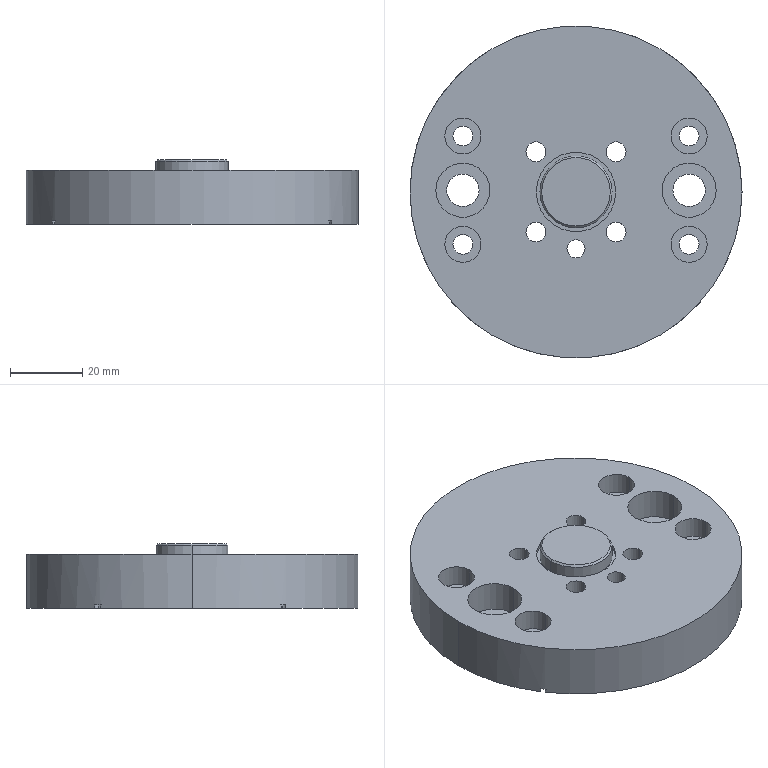Part | STEP file | ASND-0110-TPIM-020 | 1 solid | 90 faces | box 92 x 92 x 18 mm | volume 89646 mm3 | cylinder 62 | plane 26 | cone 2 | commonest cylinder face diameters 5.5 x16 10 x16 2 x14 9 x4 15 x4 5 x2